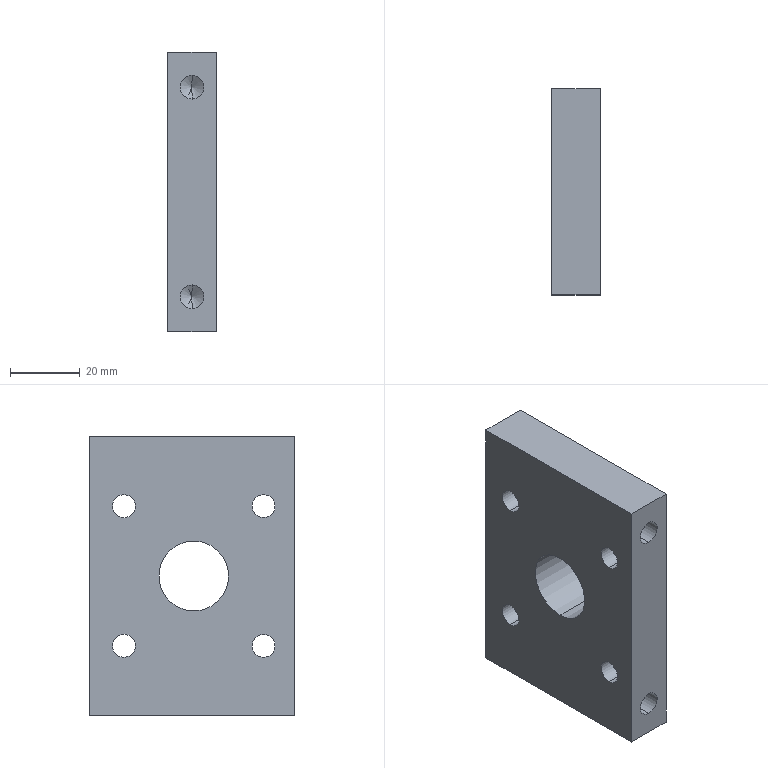Part | STEP file | 1 solid | 36 faces | box 14 x 59 x 80 mm | volume 56725 mm3 | cylinder 22 | plane 10 | cone 4 | commonest cylinder face diameters 6.6 x8 11 x8 6.8 x4 20 x2